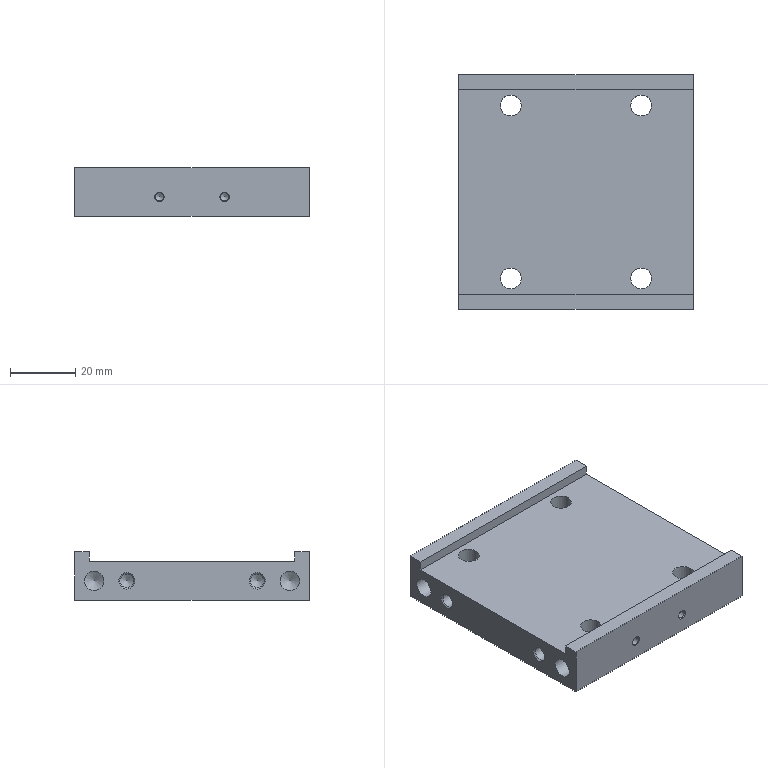Part | NX | 1 solid | 54 faces | box 72 x 72 x 15 mm | volume 58991 mm3 | cylinder 20 | cone 20 | plane 14 | commonest cylinder face diameters 2.5 x4 4.2 x4 6 x4 6.4 x4 11 x4
STEP:
#1=CARTESIAN_POINT('',(25.5,-26.5,0.));
#2=VERTEX_POINT('',#1);
#3=CARTESIAN_POINT('',(20.,-26.5,0.));
#4=DIRECTION('',(0.,0.,-1.));
#5=DIRECTION('',(1.,0.,0.));
#6=AXIS2_PLACEMENT_3D('',#3,#4,#5);
#7=CIRCLE('',#6,5.5);
#8=EDGE_CURVE('',#2,#2,#7,.T.);
#9=ORIENTED_EDGE('',*,*,#8,.F.);
#10=EDGE_LOOP('',(#9));
#11=FACE_BOUND('',#10,.T.);
#12=CARTESIAN_POINT('',(-36.,-36.,0.));
#13=VERTEX_POINT('',#12);
#14=CARTESIAN_POINT('',(-36.,36.,0.));
#15=VERTEX_POINT('',#14);
#16=CARTESIAN_POINT('',(-36.,-36.,0.));
#17=DIRECTION('',(0.,1.,0.));
#18=VECTOR('',#17,1.);
#19=LINE('',#16,#18);
#20=EDGE_CURVE('',#13,#15,#19,.T.);
#21=ORIENTED_EDGE('',*,*,#20,.T.);
#22=CARTESIAN_POINT('',(36.,36.,0.));
#23=VERTEX_POINT('',#22);
#24=CARTESIAN_POINT('',(36.,36.,0.));
#25=DIRECTION('',(-1.,0.,0.));
#26=VECTOR('',#25,1.);
#27=LINE('',#24,#26);
#28=EDGE_CURVE('',#23,#15,#27,.T.);
#29=ORIENTED_EDGE('',*,*,#28,.F.);
#30=CARTESIAN_POINT('',(36.,-36.,0.));
#31=VERTEX_POINT('',#30);
#32=CARTESIAN_POINT('',(36.,-36.,0.));
#33=DIRECTION('',(0.,1.,0.));
#34=VECTOR('',#33,1.);
#35=LINE('',#32,#34);
#36=EDGE_CURVE('',#31,#23,#35,.T.);
#37=ORIENTED_EDGE('',*,*,#36,.F.);
#38=CARTESIAN_POINT('',(36.,-36.,0.));
#39=DIRECTION('',(-1.,0.,0.));
#40=VECTOR('',#39,1.);
#41=LINE('',#38,#40);
#42=EDGE_CURVE('',#31,#13,#41,.T.);
#43=ORIENTED_EDGE('',*,*,#42,.T.);
#44=EDGE_LOOP('',(#21,#29,#37,#43));
#45=FACE_BOUND('',#44,.T.);
#46=CARTESIAN_POINT('',(-14.5,-26.5,0.));
#47=VERTEX_POINT('',#46);
#48=CARTESIAN_POINT('',(-20.,-26.5,0.));
#49=DIRECTION('',(0.,0.,1.));
#50=DIRECTION('',(1.,0.,0.));
#51=AXIS2_PLACEMENT_3D('',#48,#49,#50);
#52=CIRCLE('',#51,5.5);
#53=EDGE_CURVE('',#47,#47,#52,.T.);
#54=ORIENTED_EDGE('',*,*,#53,.T.);
#55=EDGE_LOOP('',(#54));
#56=FACE_BOUND('',#55,.T.);
#57=CARTESIAN_POINT('',(25.5,26.5,0.));
#58=VERTEX_POINT('',#57);
#59=CARTESIAN_POINT('',(20.,26.5,0.));
#60=DIRECTION('',(0.,0.,-1.));
#61=DIRECTION('',(1.,0.,0.));
#62=AXIS2_PLACEMENT_3D('',#59,#60,#61);
#63=CIRCLE('',#62,5.5);
#64=EDGE_CURVE('',#58,#58,#63,.T.);
#65=ORIENTED_EDGE('',*,*,#64,.F.);
#66=EDGE_LOOP('',(#65));
#67=FACE_BOUND('',#66,.T.);
#68=CARTESIAN_POINT('',(-14.5,26.5,0.));
#69=VERTEX_POINT('',#68);
#70=CARTESIAN_POINT('',(-20.,26.5,0.));
#71=DIRECTION('',(0.,0.,-1.));
#72=DIRECTION('',(1.,0.,0.));
#73=AXIS2_PLACEMENT_3D('',#70,#71,#72);
#74=CIRCLE('',#73,5.5);
#75=EDGE_CURVE('',#69,#69,#74,.T.);
#76=ORIENTED_EDGE('',*,*,#75,.F.);
#77=EDGE_LOOP('',(#76));
#78=FACE_BOUND('',#77,.T.);
#79=CARTESIAN_POINT('',(36.,-36.,0.));
#80=DIRECTION('',(0.,0.,1.));
#81=DIRECTION('',(-1.,0.,0.));
#82=AXIS2_PLACEMENT_3D('',#79,#80,#81);
#83=PLANE('',#82);
#84=ADVANCED_FACE('',(#11,#45,#56,#67,#78),#83,.F.);
#85=CARTESIAN_POINT('',(16.8,26.5,12.));
#86=VERTEX_POINT('',#85);
#87=CARTESIAN_POINT('',(20.,26.5,12.));
#88=DIRECTION('',(0.,0.,-1.));
#89=DIRECTION('',(-1.,0.,0.));
#90=AXIS2_PLACEMENT_3D('',#87,#88,#89);
#91=CIRCLE('',#90,3.2);
#92=EDGE_CURVE('',#86,#86,#91,.T.);
#93=ORIENTED_EDGE('',*,*,#92,.F.);
#94=EDGE_LOOP('',(#93));
#95=FACE_BOUND('',#94,.T.);
#96=CARTESIAN_POINT('',(16.8,26.5,6.8));
#97=VERTEX_POINT('',#96);
#98=CARTESIAN_POINT('',(20.,26.5,6.8));
#99=DIRECTION('',(0.,0.,1.));
#100=DIRECTION('',(-1.,0.,0.));
#101=AXIS2_PLACEMENT_3D('',#98,#99,#100);
#102=CIRCLE('',#101,3.2);
#103=EDGE_CURVE('',#97,#97,#102,.T.);
#104=ORIENTED_EDGE('',*,*,#103,.F.);
#105=EDGE_LOOP('',(#104));
#106=FACE_BOUND('',#105,.T.);
#107=CARTESIAN_POINT('',(20.,26.5,-60.));
#108=DIRECTION('',(0.,0.,1.));
#109=DIRECTION('',(-1.,0.,0.));
#110=AXIS2_PLACEMENT_3D('',#107,#108,#109);
#111=CYLINDRICAL_SURFACE('',#110,3.2);
#112=ADVANCED_FACE('',(#95,#106),#111,.F.);
#113=CARTESIAN_POINT('',(16.8,-26.5,12.));
#114=VERTEX_POINT('',#113);
#115=CARTESIAN_POINT('',(20.,-26.5,12.));
#116=DIRECTION('',(0.,0.,-1.));
#117=DIRECTION('',(-1.,0.,0.));
#118=AXIS2_PLACEMENT_3D('',#115,#116,#117);
#119=CIRCLE('',#118,3.2);
#120=EDGE_CURVE('',#114,#114,#119,.T.);
#121=ORIENTED_EDGE('',*,*,#120,.F.);
#122=EDGE_LOOP('',(#121));
#123=FACE_BOUND('',#122,.T.);
#124=CARTESIAN_POINT('',(16.8,-26.5,6.8));
#125=VERTEX_POINT('',#124);
#126=CARTESIAN_POINT('',(20.,-26.5,6.8));
#127=DIRECTION('',(0.,0.,1.));
#128=DIRECTION('',(-1.,0.,0.));
#129=AXIS2_PLACEMENT_3D('',#126,#127,#128);
#130=CIRCLE('',#129,3.2);
#131=EDGE_CURVE('',#125,#125,#130,.T.);
#132=ORIENTED_EDGE('',*,*,#131,.F.);
#133=EDGE_LOOP('',(#132));
#134=FACE_BOUND('',#133,.T.);
#135=CARTESIAN_POINT('',(20.,-26.5,-60.));
#136=DIRECTION('',(0.,0.,1.));
#137=DIRECTION('',(-1.,0.,0.));
#138=AXIS2_PLACEMENT_3D('',#135,#136,#137);
#139=CYLINDRICAL_SURFACE('',#138,3.2);
#140=ADVANCED_FACE('',(#123,#134),#139,.F.);
#141=CARTESIAN_POINT('',(-23.2,26.5,12.));
#142=VERTEX_POINT('',#141);
#143=CARTESIAN_POINT('',(-20.,26.5,12.));
#144=DIRECTION('',(0.,0.,-1.));
#145=DIRECTION('',(-1.,0.,0.));
#146=AXIS2_PLACEMENT_3D('',#143,#144,#145);
#147=CIRCLE('',#146,3.2);
#148=EDGE_CURVE('',#142,#142,#147,.T.);
#149=ORIENTED_EDGE('',*,*,#148,.F.);
#150=EDGE_LOOP('',(#149));
#151=FACE_BOUND('',#150,.T.);
#152=CARTESIAN_POINT('',(-23.2,26.5,6.8));
#153=VERTEX_POINT('',#152);
#154=CARTESIAN_POINT('',(-20.,26.5,6.8));
#155=DIRECTION('',(0.,0.,1.));
#156=DIRECTION('',(-1.,0.,0.));
#157=AXIS2_PLACEMENT_3D('',#154,#155,#156);
#158=CIRCLE('',#157,3.2);
#159=EDGE_CURVE('',#153,#153,#158,.T.);
#160=ORIENTED_EDGE('',*,*,#159,.F.);
#161=EDGE_LOOP('',(#160));
#162=FACE_BOUND('',#161,.T.);
#163=CARTESIAN_POINT('',(-20.,26.5,-60.));
#164=DIRECTION('',(0.,0.,1.));
#165=DIRECTION('',(-1.,0.,0.));
#166=AXIS2_PLACEMENT_3D('',#163,#164,#165);
#167=CYLINDRICAL_SURFACE('',#166,3.2);
#168=ADVANCED_FACE('',(#151,#162),#167,.F.);
#169=CARTESIAN_POINT('',(-23.2,-26.5,12.));
#170=VERTEX_POINT('',#169);
#171=CARTESIAN_POINT('',(-20.,-26.5,12.));
#172=DIRECTION('',(0.,0.,1.));
#173=DIRECTION('',(-1.,0.,0.));
#174=AXIS2_PLACEMENT_3D('',#171,#172,#173);
#175=CIRCLE('',#174,3.2);
#176=EDGE_CURVE('',#170,#170,#175,.T.);
#177=ORIENTED_EDGE('',*,*,#176,.F.);
#178=EDGE_LOOP('',(#177));
#179=FACE_BOUND('',#178,.T.);
#180=CARTESIAN_POINT('',(-36.,31.5,12.));
#181=VERTEX_POINT('',#180);
#182=CARTESIAN_POINT('',(-36.,-31.5,12.));
#183=VERTEX_POINT('',#182);
#184=CARTESIAN_POINT('',(-36.,31.5,12.));
#185=DIRECTION('',(0.,-1.,0.));
#186=VECTOR('',#185,1.);
#187=LINE('',#184,#186);
#188=EDGE_CURVE('',#181,#183,#187,.T.);
#189=ORIENTED_EDGE('',*,*,#188,.T.);
#190=CARTESIAN_POINT('',(36.,-31.5,12.));
#191=VERTEX_POINT('',#190);
#192=CARTESIAN_POINT('',(36.,-31.5,12.));
#193=DIRECTION('',(-1.,0.,0.));
#194=VECTOR('',#193,1.);
#195=LINE('',#192,#194);
#196=EDGE_CURVE('',#191,#183,#195,.T.);
#197=ORIENTED_EDGE('',*,*,#196,.F.);
#198=CARTESIAN_POINT('',(36.,31.5,12.));
#199=VERTEX_POINT('',#198);
#200=CARTESIAN_POINT('',(36.,31.5,12.));
#201=DIRECTION('',(0.,-1.,0.));
#202=VECTOR('',#201,1.);
#203=LINE('',#200,#202);
#204=EDGE_CURVE('',#199,#191,#203,.T.);
#205=ORIENTED_EDGE('',*,*,#204,.F.);
#206=CARTESIAN_POINT('',(36.,31.5,12.));
#207=DIRECTION('',(-1.,0.,0.));
#208=VECTOR('',#207,1.);
#209=LINE('',#206,#208);
#210=EDGE_CURVE('',#199,#181,#209,.T.);
#211=ORIENTED_EDGE('',*,*,#210,.T.);
#212=EDGE_LOOP('',(#189,#197,#205,#211));
#213=FACE_BOUND('',#212,.T.);
#214=ORIENTED_EDGE('',*,*,#92,.T.);
#215=EDGE_LOOP('',(#214));
#216=FACE_BOUND('',#215,.T.);
#217=ORIENTED_EDGE('',*,*,#120,.T.);
#218=EDGE_LOOP('',(#217));
#219=FACE_BOUND('',#218,.T.);
#220=ORIENTED_EDGE('',*,*,#148,.T.);
#221=EDGE_LOOP('',(#220));
#222=FACE_BOUND('',#221,.T.);
#223=CARTESIAN_POINT('',(36.,31.5,12.));
#224=DIRECTION('',(0.,0.,-1.));
#225=DIRECTION('',(1.,0.,0.));
#226=AXIS2_PLACEMENT_3D('',#223,#224,#225);
#227=PLANE('',#226);
#228=ADVANCED_FACE('',(#179,#213,#216,#219,#222),#227,.F.);
#229=CARTESIAN_POINT('',(10.,36.,4.5));
#230=VERTEX_POINT('',#229);
#231=CARTESIAN_POINT('',(10.,36.,6.));
#232=DIRECTION('',(0.,-1.,0.));
#233=DIRECTION('',(0.,0.,-1.));
#234=AXIS2_PLACEMENT_3D('',#231,#232,#233);
#235=CIRCLE('',#234,1.5);
#236=EDGE_CURVE('',#230,#230,#235,.T.);
#237=ORIENTED_EDGE('',*,*,#236,.T.);
#238=EDGE_LOOP('',(#237));
#239=FACE_BOUND('',#238,.T.);
#240=CARTESIAN_POINT('',(-10.,36.,4.5));
#241=VERTEX_POINT('',#240);
#242=CARTESIAN_POINT('',(-10.,36.,6.));
#243=DIRECTION('',(0.,-1.,0.));
#244=DIRECTION('',(0.,0.,-1.));
#245=AXIS2_PLACEMENT_3D('',#242,#243,#244);
#246=CIRCLE('',#245,1.5);
#247=EDGE_CURVE('',#241,#241,#246,.T.);
#248=ORIENTED_EDGE('',*,*,#247,.T.);
#249=EDGE_LOOP('',(#248));
#250=FACE_BOUND('',#249,.T.);
#251=CARTESIAN_POINT('',(-36.,36.,15.));
#252=VERTEX_POINT('',#251);
#253=CARTESIAN_POINT('',(-36.,36.,0.));
#254=DIRECTION('',(0.,0.,1.));
#255=VECTOR('',#254,1.);
#256=LINE('',#253,#255);
#257=EDGE_CURVE('',#15,#252,#256,.T.);
#258=ORIENTED_EDGE('',*,*,#257,.T.);
#259=CARTESIAN_POINT('',(36.,36.,15.));
#260=VERTEX_POINT('',#259);
#261=CARTESIAN_POINT('',(36.,36.,15.));
#262=DIRECTION('',(-1.,0.,0.));
#263=VECTOR('',#262,1.);
#264=LINE('',#261,#263);
#265=EDGE_CURVE('',#260,#252,#264,.T.);
#266=ORIENTED_EDGE('',*,*,#265,.F.);
#267=CARTESIAN_POINT('',(36.,36.,0.));
#268=DIRECTION('',(0.,0.,1.));
#269=VECTOR('',#268,1.);
#270=LINE('',#267,#269);
#271=EDGE_CURVE('',#23,#260,#270,.T.);
#272=ORIENTED_EDGE('',*,*,#271,.F.);
#273=ORIENTED_EDGE('',*,*,#28,.T.);
#274=EDGE_LOOP('',(#258,#266,#272,#273));
#275=FACE_BOUND('',#274,.T.);
#276=CARTESIAN_POINT('',(36.,36.,0.));
#277=DIRECTION('',(0.,-1.,0.));
#278=DIRECTION('',(0.,0.,1.));
#279=AXIS2_PLACEMENT_3D('',#276,#277,#278);
#280=PLANE('',#279);
#281=ADVANCED_FACE('',(#239,#250,#275),#280,.F.);
#282=CARTESIAN_POINT('',(-36.,31.5,15.));
#283=VERTEX_POINT('',#282);
#284=CARTESIAN_POINT('',(-36.,36.,15.));
#285=DIRECTION('',(0.,-1.,0.));
#286=VECTOR('',#285,1.);
#287=LINE('',#284,#286);
#288=EDGE_CURVE('',#252,#283,#287,.T.);
#289=ORIENTED_EDGE('',*,*,#288,.T.);
#290=CARTESIAN_POINT('',(36.,31.5,15.));
#291=VERTEX_POINT('',#290);
#292=CARTESIAN_POINT('',(36.,31.5,15.));
#293=DIRECTION('',(-1.,0.,0.));
#294=VECTOR('',#293,1.);
#295=LINE('',#292,#294);
#296=EDGE_CURVE('',#291,#283,#295,.T.);
#297=ORIENTED_EDGE('',*,*,#296,.F.);
#298=CARTESIAN_POINT('',(36.,36.,15.));
#299=DIRECTION('',(0.,-1.,0.));
#300=VECTOR('',#299,1.);
#301=LINE('',#298,#300);
#302=EDGE_CURVE('',#260,#291,#301,.T.);
#303=ORIENTED_EDGE('',*,*,#302,.F.);
#304=ORIENTED_EDGE('',*,*,#265,.T.);
#305=EDGE_LOOP('',(#289,#297,#303,#304));
#306=FACE_OUTER_BOUND('',#305,.T.);
#307=CARTESIAN_POINT('',(36.,36.,15.));
#308=DIRECTION('',(0.,0.,-1.));
#309=DIRECTION('',(1.,0.,0.));
#310=AXIS2_PLACEMENT_3D('',#307,#308,#309);
#311=PLANE('',#310);
#312=ADVANCED_FACE('',(#306),#311,.F.);
#313=CARTESIAN_POINT('',(-36.,31.5,15.));
#314=DIRECTION('',(0.,0.,-1.));
#315=VECTOR('',#314,1.);
#316=LINE('',#313,#315);
#317=EDGE_CURVE('',#283,#181,#316,.T.);
#318=ORIENTED_EDGE('',*,*,#317,.T.);
#319=ORIENTED_EDGE('',*,*,#210,.F.);
#320=CARTESIAN_POINT('',(36.,31.5,15.));
#321=DIRECTION('',(0.,0.,-1.));
#322=VECTOR('',#321,1.);
#323=LINE('',#320,#322);
#324=EDGE_CURVE('',#291,#199,#323,.T.);
#325=ORIENTED_EDGE('',*,*,#324,.F.);
#326=ORIENTED_EDGE('',*,*,#296,.T.);
#327=EDGE_LOOP('',(#318,#319,#325,#326));
#328=FACE_OUTER_BOUND('',#327,.T.);
#329=CARTESIAN_POINT('',(36.,31.5,15.));
#330=DIRECTION('',(0.,1.,0.));
#331=DIRECTION('',(0.,0.,-1.));
#332=AXIS2_PLACEMENT_3D('',#329,#330,#331);
#333=PLANE('',#332);
#334=ADVANCED_FACE('',(#328),#333,.F.);
#335=CARTESIAN_POINT('',(-36.,-31.5,15.));
#336=VERTEX_POINT('',#335);
#337=CARTESIAN_POINT('',(-36.,-31.5,12.));
#338=DIRECTION('',(0.,0.,1.));
#339=VECTOR('',#338,1.);
#340=LINE('',#337,#339);
#341=EDGE_CURVE('',#183,#336,#340,.T.);
#342=ORIENTED_EDGE('',*,*,#341,.T.);
#343=CARTESIAN_POINT('',(36.,-31.5,15.));
#344=VERTEX_POINT('',#343);
#345=CARTESIAN_POINT('',(36.,-31.5,15.));
#346=DIRECTION('',(-1.,0.,0.));
#347=VECTOR('',#346,1.);
#348=LINE('',#345,#347);
#349=EDGE_CURVE('',#344,#336,#348,.T.);
#350=ORIENTED_EDGE('',*,*,#349,.F.);
#351=CARTESIAN_POINT('',(36.,-31.5,12.));
#352=DIRECTION('',(0.,0.,1.));
#353=VECTOR('',#352,1.);
#354=LINE('',#351,#353);
#355=EDGE_CURVE('',#191,#344,#354,.T.);
#356=ORIENTED_EDGE('',*,*,#355,.F.);
#357=ORIENTED_EDGE('',*,*,#196,.T.);
#358=EDGE_LOOP('',(#342,#350,#356,#357));
#359=FACE_OUTER_BOUND('',#358,.T.);
#360=CARTESIAN_POINT('',(36.,-31.5,12.));
#361=DIRECTION('',(0.,-1.,0.));
#362=DIRECTION('',(0.,0.,1.));
#363=AXIS2_PLACEMENT_3D('',#360,#361,#362);
#364=PLANE('',#363);
#365=ADVANCED_FACE('',(#359),#364,.F.);
#366=CARTESIAN_POINT('',(-36.,-36.,15.));
#367=VERTEX_POINT('',#366);
#368=CARTESIAN_POINT('',(-36.,-31.5,15.));
#369=DIRECTION('',(0.,-1.,0.));
#370=VECTOR('',#369,1.);
#371=LINE('',#368,#370);
#372=EDGE_CURVE('',#336,#367,#371,.T.);
#373=ORIENTED_EDGE('',*,*,#372,.T.);
#374=CARTESIAN_POINT('',(36.,-36.,15.));
#375=VERTEX_POINT('',#374);
#376=CARTESIAN_POINT('',(36.,-36.,15.));
#377=DIRECTION('',(-1.,0.,0.));
#378=VECTOR('',#377,1.);
#379=LINE('',#376,#378);
#380=EDGE_CURVE('',#375,#367,#379,.T.);
#381=ORIENTED_EDGE('',*,*,#380,.F.);
#382=CARTESIAN_POINT('',(36.,-31.5,15.));
#383=DIRECTION('',(0.,-1.,0.));
#384=VECTOR('',#383,1.);
#385=LINE('',#382,#384);
#386=EDGE_CURVE('',#344,#375,#385,.T.);
#387=ORIENTED_EDGE('',*,*,#386,.F.);
#388=ORIENTED_EDGE('',*,*,#349,.T.);
#389=EDGE_LOOP('',(#373,#381,#387,#388));
#390=FACE_OUTER_BOUND('',#389,.T.);
#391=CARTESIAN_POINT('',(36.,-31.5,15.));
#392=DIRECTION('',(0.,0.,-1.));
#393=DIRECTION('',(1.,0.,0.));
#394=AXIS2_PLACEMENT_3D('',#391,#392,#393);
#395=PLANE('',#394);
#396=ADVANCED_FACE('',(#390),#395,.F.);
#397=CARTESIAN_POINT('',(10.,-36.,7.5));
#398=VERTEX_POINT('',#397);
#399=CARTESIAN_POINT('',(10.,-36.,6.));
#400=DIRECTION('',(0.,1.,0.));
#401=DIRECTION('',(0.,0.,1.));
#402=AXIS2_PLACEMENT_3D('',#399,#400,#401);
#403=CIRCLE('',#402,1.5);
#404=EDGE_CURVE('',#398,#398,#403,.T.);
#405=ORIENTED_EDGE('',*,*,#404,.T.);
#406=EDGE_LOOP('',(#405));
#407=FACE_BOUND('',#406,.T.);
#408=CARTESIAN_POINT('',(-10.,-36.,7.5));
#409=VERTEX_POINT('',#408);
#410=CARTESIAN_POINT('',(-10.,-36.,6.));
#411=DIRECTION('',(0.,1.,0.));
#412=DIRECTION('',(0.,0.,1.));
#413=AXIS2_PLACEMENT_3D('',#410,#411,#412);
#414=CIRCLE('',#413,1.5);
#415=EDGE_CURVE('',#409,#409,#414,.T.);
#416=ORIENTED_EDGE('',*,*,#415,.T.);
#417=EDGE_LOOP('',(#416));
#418=FACE_BOUND('',#417,.T.);
#419=CARTESIAN_POINT('',(-36.,-36.,15.));
#420=DIRECTION('',(0.,0.,-1.));
#421=VECTOR('',#420,1.);
#422=LINE('',#419,#421);
#423=EDGE_CURVE('',#367,#13,#422,.T.);
#424=ORIENTED_EDGE('',*,*,#423,.T.);
#425=ORIENTED_EDGE('',*,*,#42,.F.);
#426=CARTESIAN_POINT('',(36.,-36.,15.));
#427=DIRECTION('',(0.,0.,-1.));
#428=VECTOR('',#427,1.);
#429=LINE('',#426,#428);
#430=EDGE_CURVE('',#375,#31,#429,.T.);
#431=ORIENTED_EDGE('',*,*,#430,.F.);
#432=ORIENTED_EDGE('',*,*,#380,.T.);
#433=EDGE_LOOP('',(#424,#425,#431,#432));
#434=FACE_BOUND('',#433,.T.);
#435=CARTESIAN_POINT('',(36.,-36.,15.));
#436=DIRECTION('',(0.,1.,0.));
#437=DIRECTION('',(0.,0.,-1.));
#438=AXIS2_PLACEMENT_3D('',#435,#436,#437);
#439=PLANE('',#438);
#440=ADVANCED_FACE('',(#407,#418,#434),#439,.F.);
#441=CARTESIAN_POINT('',(36.,20.,3.5));
#442=VERTEX_POINT('',#441);
#443=CARTESIAN_POINT('',(36.,20.,6.));
#444=DIRECTION('',(-1.,0.,0.));
#445=DIRECTION('',(0.,0.,-1.));
#446=AXIS2_PLACEMENT_3D('',#443,#444,#445);
#447=CIRCLE('',#446,2.5);
#448=EDGE_CURVE('',#442,#442,#447,.T.);
#449=ORIENTED_EDGE('',*,*,#448,.T.);
#450=EDGE_LOOP('',(#449));
#451=FACE_BOUND('',#450,.T.);
#452=CARTESIAN_POINT('',(36.,-20.,3.5));
#453=VERTEX_POINT('',#452);
#454=CARTESIAN_POINT('',(36.,-20.,6.));
#455=DIRECTION('',(-1.,0.,0.));
#456=DIRECTION('',(0.,0.,-1.));
#457=AXIS2_PLACEMENT_3D('',#454,#455,#456);
#458=CIRCLE('',#457,2.5);
#459=EDGE_CURVE('',#453,#453,#458,.T.);
#460=ORIENTED_EDGE('',*,*,#459,.T.);
#461=EDGE_LOOP('',(#460));
#462=FACE_BOUND('',#461,.T.);
#463=CARTESIAN_POINT('',(36.,30.,9.));
#464=VERTEX_POINT('',#463);
#465=CARTESIAN_POINT('',(36.,30.,6.));
#466=DIRECTION('',(-1.,0.,0.));
#467=DIRECTION('',(0.,0.,1.));
#468=AXIS2_PLACEMENT_3D('',#465,#466,#467);
#469=CIRCLE('',#468,3.);
#470=EDGE_CURVE('',#464,#464,#469,.T.);
#471=ORIENTED_EDGE('',*,*,#470,.T.);
#472=EDGE_LOOP('',(#471));
#473=FACE_BOUND('',#472,.T.);
#474=CARTESIAN_POINT('',(36.,-30.,9.));
#475=VERTEX_POINT('',#474);
#476=CARTESIAN_POINT('',(36.,-30.,6.));
#477=DIRECTION('',(-1.,0.,0.));
#478=DIRECTION('',(0.,0.,1.));
#479=AXIS2_PLACEMENT_3D('',#476,#477,#478);
#480=CIRCLE('',#479,3.);
#481=EDGE_CURVE('',#475,#475,#480,.T.);
#482=ORIENTED_EDGE('',*,*,#481,.T.);
#483=EDGE_LOOP('',(#482));
#484=FACE_BOUND('',#483,.T.);
#485=ORIENTED_EDGE('',*,*,#36,.T.);
#486=ORIENTED_EDGE('',*,*,#271,.T.);
#487=ORIENTED_EDGE('',*,*,#302,.T.);
#488=ORIENTED_EDGE('',*,*,#324,.T.);
#489=ORIENTED_EDGE('',*,*,#204,.T.);
#490=ORIENTED_EDGE('',*,*,#355,.T.);
#491=ORIENTED_EDGE('',*,*,#386,.T.);
#492=ORIENTED_EDGE('',*,*,#430,.T.);
#493=EDGE_LOOP('',(#485,#486,#487,#488,#489,#490,#491,#492));
#494=FACE_BOUND('',#493,.T.);
#495=CARTESIAN_POINT('',(36.,0.,0.));
#496=DIRECTION('',(1.,0.,0.));
#497=DIRECTION('',(0.,0.,1.));
#498=AXIS2_PLACEMENT_3D('',#495,#496,#497);
#499=PLANE('',#498);
#500=ADVANCED_FACE('',(#451,#462,#473,#484,#494),#499,.T.);
#501=CARTESIAN_POINT('',(-36.,20.,3.5));
#502=VERTEX_POINT('',#501);
#503=CARTESIAN_POINT('',(-36.,20.,6.));
#504=DIRECTION('',(1.,0.,0.));
#505=DIRECTION('',(0.,0.,-1.));
#506=AXIS2_PLACEMENT_3D('',#503,#504,#505);
#507=CIRCLE('',#506,2.5);
#508=EDGE_CURVE('',#502,#502,#507,.T.);
#509=ORIENTED_EDGE('',*,*,#508,.T.);
#510=EDGE_LOOP('',(#509));
#511=FACE_BOUND('',#510,.T.);
#512=CARTESIAN_POINT('',(-36.,-20.,3.5));
#513=VERTEX_POINT('',#512);
#514=CARTESIAN_POINT('',(-36.,-20.,6.));
#515=DIRECTION('',(1.,0.,0.));
#516=DIRECTION('',(0.,0.,-1.));
#517=AXIS2_PLACEMENT_3D('',#514,#515,#516);
#518=CIRCLE('',#517,2.5);
#519=EDGE_CURVE('',#513,#513,#518,.T.);
#520=ORIENTED_EDGE('',*,*,#519,.T.);
#521=EDGE_LOOP('',(#520));
#522=FACE_BOUND('',#521,.T.);
#523=CARTESIAN_POINT('',(-36.,30.,3.));
#524=VERTEX_POINT('',#523);
#525=CARTESIAN_POINT('',(-36.,30.,6.));
#526=DIRECTION('',(1.,0.,0.));
#527=DIRECTION('',(0.,0.,-1.));
#528=AXIS2_PLACEMENT_3D('',#525,#526,#527);
#529=CIRCLE('',#528,3.);
#530=EDGE_CURVE('',#524,#524,#529,.T.);
#531=ORIENTED_EDGE('',*,*,#530,.T.);
#532=EDGE_LOOP('',(#531));
#533=FACE_BOUND('',#532,.T.);
#534=CARTESIAN_POINT('',(-36.,-30.,3.));
#535=VERTEX_POINT('',#534);
#536=CARTESIAN_POINT('',(-36.,-30.,6.));
#537=DIRECTION('',(1.,0.,0.));
#538=DIRECTION('',(0.,0.,-1.));
#539=AXIS2_PLACEMENT_3D('',#536,#537,#538);
#540=CIRCLE('',#539,3.);
#541=EDGE_CURVE('',#535,#535,#540,.T.);
#542=ORIENTED_EDGE('',*,*,#541,.T.);
#543=EDGE_LOOP('',(#542));
#544=FACE_BOUND('',#543,.T.);
#545=ORIENTED_EDGE('',*,*,#20,.F.);
#546=ORIENTED_EDGE('',*,*,#423,.F.);
#547=ORIENTED_EDGE('',*,*,#372,.F.);
#548=ORIENTED_EDGE('',*,*,#341,.F.);
#549=ORIENTED_EDGE('',*,*,#188,.F.);
#550=ORIENTED_EDGE('',*,*,#317,.F.);
#551=ORIENTED_EDGE('',*,*,#288,.F.);
#552=ORIENTED_EDGE('',*,*,#257,.F.);
#553=EDGE_LOOP('',(#545,#546,#547,#548,#549,#550,#551,#552));
#554=FACE_BOUND('',#553,.T.);
#555=CARTESIAN_POINT('',(-36.,0.,0.));
#556=DIRECTION('',(1.,0.,0.));
#557=DIRECTION('',(0.,0.,1.));
#558=AXIS2_PLACEMENT_3D('',#555,#556,#557);
#559=PLANE('',#558);
#560=ADVANCED_FACE('',(#511,#522,#533,#544,#554),#559,.F.);
#561=CARTESIAN_POINT('',(-16.8,-26.5,6.8));
#562=VERTEX_POINT('',#561);
#563=CARTESIAN_POINT('',(-20.,-26.5,6.8));
#564=DIRECTION('',(0.,0.,-1.));
#565=DIRECTION('',(1.,0.,0.));
#566=AXIS2_PLACEMENT_3D('',#563,#564,#565);
#567=CIRCLE('',#566,3.2);
#568=EDGE_CURVE('',#562,#562,#567,.T.);
#569=ORIENTED_EDGE('',*,*,#568,.T.);
#570=EDGE_LOOP('',(#569));
#571=FACE_BOUND('',#570,.T.);
#572=ORIENTED_EDGE('',*,*,#176,.T.);
#573=EDGE_LOOP('',(#572));
#574=FACE_BOUND('',#573,.T.);
#575=CARTESIAN_POINT('',(-20.,-26.5,-60.));
#576=DIRECTION('',(0.,0.,1.));
#577=DIRECTION('',(-1.,0.,0.));
#578=AXIS2_PLACEMENT_3D('',#575,#576,#577);
#579=CYLINDRICAL_SURFACE('',#578,3.2);
#580=ADVANCED_FACE('',(#571,#574),#579,.F.);
#581=CARTESIAN_POINT('',(-25.5,26.5,6.8));
#582=VERTEX_POINT('',#581);
#583=CARTESIAN_POINT('',(-20.,26.5,6.8));
#584=DIRECTION('',(0.,0.,-1.));
#585=DIRECTION('',(-1.,0.,0.));
#586=AXIS2_PLACEMENT_3D('',#583,#584,#585);
#587=CIRCLE('',#586,5.5);
#588=EDGE_CURVE('',#582,#582,#587,.T.);
#589=ORIENTED_EDGE('',*,*,#588,.F.);
#590=EDGE_LOOP('',(#589));
#591=FACE_BOUND('',#590,.T.);
#592=ORIENTED_EDGE('',*,*,#75,.T.);
#593=EDGE_LOOP('',(#592));
#594=FACE_BOUND('',#593,.T.);
#595=CARTESIAN_POINT('',(-20.,26.5,-60.));
#596=DIRECTION('',(0.,0.,1.));
#597=DIRECTION('',(-1.,0.,0.));
#598=AXIS2_PLACEMENT_3D('',#595,#596,#597);
#599=CYLINDRICAL_SURFACE('',#598,5.5);
#600=ADVANCED_FACE('',(#591,#594),#599,.F.);
#601=ORIENTED_EDGE('',*,*,#159,.T.);
#602=EDGE_LOOP('',(#601));
#603=FACE_BOUND('',#602,.T.);
#604=ORIENTED_EDGE('',*,*,#588,.T.);
#605=EDGE_LOOP('',(#604));
#606=FACE_BOUND('',#605,.T.);
#607=CARTESIAN_POINT('',(-20.,26.5,6.8));
#608=DIRECTION('',(0.,0.,-1.));
#609=DIRECTION('',(1.,0.,0.));
#610=AXIS2_PLACEMENT_3D('',#607,#608,#609);
#611=PLANE('',#610);
#612=ADVANCED_FACE('',(#603,#606),#611,.T.);
#613=CARTESIAN_POINT('',(14.5,-26.5,6.8));
#614=VERTEX_POINT('',#613);
#615=CARTESIAN_POINT('',(20.,-26.5,6.8));
#616=DIRECTION('',(0.,0.,-1.));
#617=DIRECTION('',(-1.,0.,0.));
#618=AXIS2_PLACEMENT_3D('',#615,#616,#617);
#619=CIRCLE('',#618,5.5);
#620=EDGE_CURVE('',#614,#614,#619,.T.);
#621=ORIENTED_EDGE('',*,*,#620,.F.);
#622=EDGE_LOOP('',(#621));
#623=FACE_BOUND('',#622,.T.);
#624=ORIENTED_EDGE('',*,*,#8,.T.);
#625=EDGE_LOOP('',(#624));
#626=FACE_BOUND('',#625,.T.);
#627=CARTESIAN_POINT('',(20.,-26.5,-60.));
#628=DIRECTION('',(0.,0.,1.));
#629=DIRECTION('',(-1.,0.,0.));
#630=AXIS2_PLACEMENT_3D('',#627,#628,#629);
#631=CYLINDRICAL_SURFACE('',#630,5.5);
#632=ADVANCED_FACE('',(#623,#626),#631,.F.);
#633=ORIENTED_EDGE('',*,*,#131,.T.);
#634=EDGE_LOOP('',(#633));
#635=FACE_BOUND('',#634,.T.);
#636=ORIENTED_EDGE('',*,*,#620,.T.);
#637=EDGE_LOOP('',(#636));
#638=FACE_BOUND('',#637,.T.);
#639=CARTESIAN_POINT('',(20.,-26.5,6.8));
#640=DIRECTION('',(0.,0.,-1.));
#641=DIRECTION('',(1.,0.,0.));
#642=AXIS2_PLACEMENT_3D('',#639,#640,#641);
#643=PLANE('',#642);
#644=ADVANCED_FACE('',(#635,#638),#643,.T.);
#645=CARTESIAN_POINT('',(14.5,26.5,6.8));
#646=VERTEX_POINT('',#645);
#647=CARTESIAN_POINT('',(20.,26.5,6.8));
#648=DIRECTION('',(0.,0.,-1.));
#649=DIRECTION('',(-1.,0.,0.));
#650=AXIS2_PLACEMENT_3D('',#647,#648,#649);
#651=CIRCLE('',#650,5.5);
#652=EDGE_CURVE('',#646,#646,#651,.T.);
#653=ORIENTED_EDGE('',*,*,#652,.F.);
#654=EDGE_LOOP('',(#653));
#655=FACE_BOUND('',#654,.T.);
#656=ORIENTED_EDGE('',*,*,#64,.T.);
#657=EDGE_LOOP('',(#656));
#658=FACE_BOUND('',#657,.T.);
#659=CARTESIAN_POINT('',(20.,26.5,-60.));
#660=DIRECTION('',(0.,0.,1.));
#661=DIRECTION('',(-1.,0.,0.));
#662=AXIS2_PLACEMENT_3D('',#659,#660,#661);
#663=CYLINDRICAL_SURFACE('',#662,5.5);
#664=ADVANCED_FACE('',(#655,#658),#663,.F.);
#665=ORIENTED_EDGE('',*,*,#103,.T.);
#666=EDGE_LOOP('',(#665));
#667=FACE_BOUND('',#666,.T.);
#668=ORIENTED_EDGE('',*,*,#652,.T.);
#669=EDGE_LOOP('',(#668));
#670=FACE_BOUND('',#669,.T.);
#671=CARTESIAN_POINT('',(20.,26.5,6.8));
#672=DIRECTION('',(0.,0.,-1.));
#673=DIRECTION('',(1.,0.,0.));
#674=AXIS2_PLACEMENT_3D('',#671,#672,#673);
#675=PLANE('',#674);
#676=ADVANCED_FACE('',(#667,#670),#675,.T.);
#677=CARTESIAN_POINT('',(-25.5,-26.5,6.8));
#678=VERTEX_POINT('',#677);
#679=CARTESIAN_POINT('',(-20.,-26.5,6.8));
#680=DIRECTION('',(0.,0.,1.));
#681=DIRECTION('',(-1.,0.,0.));
#682=AXIS2_PLACEMENT_3D('',#679,#680,#681);
#683=CIRCLE('',#682,5.5);
#684=EDGE_CURVE('',#678,#678,#683,.T.);
#685=ORIENTED_EDGE('',*,*,#684,.T.);
#686=EDGE_LOOP('',(#685));
#687=FACE_BOUND('',#686,.T.);
#688=ORIENTED_EDGE('',*,*,#53,.F.);
#689=EDGE_LOOP('',(#688));
#690=FACE_BOUND('',#689,.T.);
#691=CARTESIAN_POINT('',(-20.,-26.5,-60.));
#692=DIRECTION('',(0.,0.,1.));
#693=DIRECTION('',(-1.,0.,0.));
#694=AXIS2_PLACEMENT_3D('',#691,#692,#693);
#695=CYLINDRICAL_SURFACE('',#694,5.5);
#696=ADVANCED_FACE('',(#687,#690),#695,.F.);
#697=ORIENTED_EDGE('',*,*,#684,.F.);
#698=EDGE_LOOP('',(#697));
#699=FACE_BOUND('',#698,.T.);
#700=ORIENTED_EDGE('',*,*,#568,.F.);
#701=EDGE_LOOP('',(#700));
#702=FACE_BOUND('',#701,.T.);
#703=CARTESIAN_POINT('',(-20.,-26.5,6.8));
#704=DIRECTION('',(0.,0.,1.));
#705=DIRECTION('',(-1.,0.,0.));
#706=AXIS2_PLACEMENT_3D('',#703,#704,#705);
#707=PLANE('',#706);
#708=ADVANCED_FACE('',(#699,#702),#707,.F.);
#709=CARTESIAN_POINT('',(-28.,-30.,3.));
#710=VERTEX_POINT('',#709);
#711=CARTESIAN_POINT('',(-28.,-30.,6.));
#712=DIRECTION('',(-1.,0.,0.));
#713=DIRECTION('',(0.,0.,-1.));
#714=AXIS2_PLACEMENT_3D('',#711,#712,#713);
#715=CIRCLE('',#714,3.);
#716=EDGE_CURVE('',#710,#710,#715,.T.);
#717=ORIENTED_EDGE('',*,*,#716,.T.);
#718=EDGE_LOOP('',(#717));
#719=FACE_BOUND('',#718,.T.);
#720=CARTESIAN_POINT('',(-26.197,-30.,6.));
#721=VERTEX_POINT('',#720);
#722=VERTEX_LOOP('',#721);
#723=FACE_BOUND('',#722,.T.);
#724=CARTESIAN_POINT('',(-28.,-30.,6.));
#725=DIRECTION('',(-1.,0.,0.));
#726=DIRECTION('',(0.,0.,-1.));
#727=AXIS2_PLACEMENT_3D('',#724,#725,#726);
#728=CONICAL_SURFACE('',#727,3.,59.);
#729=ADVANCED_FACE('',(#719,#723),#728,.F.);
#730=ORIENTED_EDGE('',*,*,#716,.F.);
#731=EDGE_LOOP('',(#730));
#732=FACE_BOUND('',#731,.T.);
#733=ORIENTED_EDGE('',*,*,#541,.F.);
#734=EDGE_LOOP('',(#733));
#735=FACE_BOUND('',#734,.T.);
#736=CARTESIAN_POINT('',(-36.,-30.,6.));
#737=DIRECTION('',(1.,0.,0.));
#738=DIRECTION('',(0.,0.,1.));
#739=AXIS2_PLACEMENT_3D('',#736,#737,#738);
#740=CYLINDRICAL_SURFACE('',#739,3.);
#741=ADVANCED_FACE('',(#732,#735),#740,.F.);
#742=CARTESIAN_POINT('',(-28.,30.,3.));
#743=VERTEX_POINT('',#742);
#744=CARTESIAN_POINT('',(-28.,30.,6.));
#745=DIRECTION('',(-1.,0.,0.));
#746=DIRECTION('',(0.,0.,-1.));
#747=AXIS2_PLACEMENT_3D('',#744,#745,#746);
#748=CIRCLE('',#747,3.);
#749=EDGE_CURVE('',#743,#743,#748,.T.);
#750=ORIENTED_EDGE('',*,*,#749,.T.);
#751=EDGE_LOOP('',(#750));
#752=FACE_BOUND('',#751,.T.);
#753=CARTESIAN_POINT('',(-26.197,30.,6.));
#754=VERTEX_POINT('',#753);
#755=VERTEX_LOOP('',#754);
#756=FACE_BOUND('',#755,.T.);
#757=CARTESIAN_POINT('',(-28.,30.,6.));
#758=DIRECTION('',(-1.,0.,0.));
#759=DIRECTION('',(0.,0.,-1.));
#760=AXIS2_PLACEMENT_3D('',#757,#758,#759);
#761=CONICAL_SURFACE('',#760,3.,59.);
#762=ADVANCED_FACE('',(#752,#756),#761,.F.);
#763=ORIENTED_EDGE('',*,*,#749,.F.);
#764=EDGE_LOOP('',(#763));
#765=FACE_BOUND('',#764,.T.);
#766=ORIENTED_EDGE('',*,*,#530,.F.);
#767=EDGE_LOOP('',(#766));
#768=FACE_BOUND('',#767,.T.);
#769=CARTESIAN_POINT('',(-36.,30.,6.));
#770=DIRECTION('',(1.,0.,0.));
#771=DIRECTION('',(0.,0.,1.));
#772=AXIS2_PLACEMENT_3D('',#769,#770,#771);
#773=CYLINDRICAL_SURFACE('',#772,3.);
#774=ADVANCED_FACE('',(#765,#768),#773,.F.);
#775=CARTESIAN_POINT('',(-24.,-20.,3.9));
#776=VERTEX_POINT('',#775);
#777=CARTESIAN_POINT('',(-24.,-20.,6.));
#778=DIRECTION('',(-1.,0.,0.));
#779=DIRECTION('',(0.,0.,-1.));
#780=AXIS2_PLACEMENT_3D('',#777,#778,#779);
#781=CIRCLE('',#780,2.1);
#782=EDGE_CURVE('',#776,#776,#781,.T.);
#783=ORIENTED_EDGE('',*,*,#782,.T.);
#784=EDGE_LOOP('',(#783));
#785=FACE_BOUND('',#784,.T.);
#786=CARTESIAN_POINT('',(-22.738,-20.,6.));
#787=VERTEX_POINT('',#786);
#788=VERTEX_LOOP('',#787);
#789=FACE_BOUND('',#788,.T.);
#790=CARTESIAN_POINT('',(-24.,-20.,6.));
#791=DIRECTION('',(-1.,0.,0.));
#792=DIRECTION('',(0.,0.,-1.));
#793=AXIS2_PLACEMENT_3D('',#790,#791,#792);
#794=CONICAL_SURFACE('',#793,2.1,59.);
#795=ADVANCED_FACE('',(#785,#789),#794,.F.);
#796=CARTESIAN_POINT('',(-35.6,-20.,3.9));
#797=VERTEX_POINT('',#796);
#798=CARTESIAN_POINT('',(-35.6,-20.,6.));
#799=DIRECTION('',(-1.,0.,0.));
#800=DIRECTION('',(0.,0.,-1.));
#801=AXIS2_PLACEMENT_3D('',#798,#799,#800);
#802=CIRCLE('',#801,2.1);
#803=EDGE_CURVE('',#797,#797,#802,.T.);
#804=ORIENTED_EDGE('',*,*,#803,.T.);
#805=EDGE_LOOP('',(#804));
#806=FACE_BOUND('',#805,.T.);
#807=ORIENTED_EDGE('',*,*,#782,.F.);
#808=EDGE_LOOP('',(#807));
#809=FACE_BOUND('',#808,.T.);
#810=CARTESIAN_POINT('',(-36.,-20.,6.));
#811=DIRECTION('',(1.,0.,0.));
#812=DIRECTION('',(0.,0.,1.));
#813=AXIS2_PLACEMENT_3D('',#810,#811,#812);
#814=CYLINDRICAL_SURFACE('',#813,2.1);
#815=ADVANCED_FACE('',(#806,#809),#814,.F.);
#816=ORIENTED_EDGE('',*,*,#803,.F.);
#817=EDGE_LOOP('',(#816));
#818=FACE_BOUND('',#817,.T.);
#819=ORIENTED_EDGE('',*,*,#519,.F.);
#820=EDGE_LOOP('',(#819));
#821=FACE_BOUND('',#820,.T.);
#822=CARTESIAN_POINT('',(-36.,-20.,6.));
#823=DIRECTION('',(-1.,0.,0.));
#824=DIRECTION('',(0.,0.,-1.));
#825=AXIS2_PLACEMENT_3D('',#822,#823,#824);
#826=CONICAL_SURFACE('',#825,2.5,45.);
#827=ADVANCED_FACE('',(#818,#821),#826,.F.);
#828=CARTESIAN_POINT('',(-24.,20.,3.9));
#829=VERTEX_POINT('',#828);
#830=CARTESIAN_POINT('',(-24.,20.,6.));
#831=DIRECTION('',(-1.,0.,0.));
#832=DIRECTION('',(0.,0.,-1.));
#833=AXIS2_PLACEMENT_3D('',#830,#831,#832);
#834=CIRCLE('',#833,2.1);
#835=EDGE_CURVE('',#829,#829,#834,.T.);
#836=ORIENTED_EDGE('',*,*,#835,.T.);
#837=EDGE_LOOP('',(#836));
#838=FACE_BOUND('',#837,.T.);
#839=CARTESIAN_POINT('',(-22.738,20.,6.));
#840=VERTEX_POINT('',#839);
#841=VERTEX_LOOP('',#840);
#842=FACE_BOUND('',#841,.T.);
#843=CARTESIAN_POINT('',(-24.,20.,6.));
#844=DIRECTION('',(-1.,0.,0.));
#845=DIRECTION('',(0.,0.,-1.));
#846=AXIS2_PLACEMENT_3D('',#843,#844,#845);
#847=CONICAL_SURFACE('',#846,2.1,59.);
#848=ADVANCED_FACE('',(#838,#842),#847,.F.);
#849=CARTESIAN_POINT('',(-35.6,20.,3.9));
#850=VERTEX_POINT('',#849);
#851=CARTESIAN_POINT('',(-35.6,20.,6.));
#852=DIRECTION('',(-1.,0.,0.));
#853=DIRECTION('',(0.,0.,-1.));
#854=AXIS2_PLACEMENT_3D('',#851,#852,#853);
#855=CIRCLE('',#854,2.1);
#856=EDGE_CURVE('',#850,#850,#855,.T.);
#857=ORIENTED_EDGE('',*,*,#856,.T.);
#858=EDGE_LOOP('',(#857));
#859=FACE_BOUND('',#858,.T.);
#860=ORIENTED_EDGE('',*,*,#835,.F.);
#861=EDGE_LOOP('',(#860));
#862=FACE_BOUND('',#861,.T.);
#863=CARTESIAN_POINT('',(-36.,20.,6.));
#864=DIRECTION('',(1.,0.,0.));
#865=DIRECTION('',(0.,0.,1.));
#866=AXIS2_PLACEMENT_3D('',#863,#864,#865);
#867=CYLINDRICAL_SURFACE('',#866,2.1);
#868=ADVANCED_FACE('',(#859,#862),#867,.F.);
#869=ORIENTED_EDGE('',*,*,#856,.F.);
#870=EDGE_LOOP('',(#869));
#871=FACE_BOUND('',#870,.T.);
#872=ORIENTED_EDGE('',*,*,#508,.F.);
#873=EDGE_LOOP('',(#872));
#874=FACE_BOUND('',#873,.T.);
#875=CARTESIAN_POINT('',(-36.,20.,6.));
#876=DIRECTION('',(-1.,0.,0.));
#877=DIRECTION('',(0.,0.,-1.));
#878=AXIS2_PLACEMENT_3D('',#875,#876,#877);
#879=CONICAL_SURFACE('',#878,2.5,45.);
#880=ADVANCED_FACE('',(#871,#874),#879,.F.);
#881=CARTESIAN_POINT('',(-10.,24.,4.75));
#882=VERTEX_POINT('',#881);
#883=CARTESIAN_POINT('',(-10.,24.,6.));
#884=DIRECTION('',(0.,1.,0.));
#885=DIRECTION('',(0.,0.,-1.));
#886=AXIS2_PLACEMENT_3D('',#883,#884,#885);
#887=CIRCLE('',#886,1.25);
#888=EDGE_CURVE('',#882,#882,#887,.T.);
#889=ORIENTED_EDGE('',*,*,#888,.T.);
#890=EDGE_LOOP('',(#889));
#891=FACE_BOUND('',#890,.T.);
#892=CARTESIAN_POINT('',(-10.,23.249,6.));
#893=VERTEX_POINT('',#892);
#894=VERTEX_LOOP('',#893);
#895=FACE_BOUND('',#894,.T.);
#896=CARTESIAN_POINT('',(-10.,24.,6.));
#897=DIRECTION('',(0.,1.,0.));
#898=DIRECTION('',(0.,0.,-1.));
#899=AXIS2_PLACEMENT_3D('',#896,#897,#898);
#900=CONICAL_SURFACE('',#899,1.25,59.);
#901=ADVANCED_FACE('',(#891,#895),#900,.F.);
#902=CARTESIAN_POINT('',(-10.,35.75,4.75));
#903=VERTEX_POINT('',#902);
#904=CARTESIAN_POINT('',(-10.,35.75,6.));
#905=DIRECTION('',(0.,1.,0.));
#906=DIRECTION('',(0.,0.,-1.));
#907=AXIS2_PLACEMENT_3D('',#904,#905,#906);
#908=CIRCLE('',#907,1.25);
#909=EDGE_CURVE('',#903,#903,#908,.T.);
#910=ORIENTED_EDGE('',*,*,#909,.T.);
#911=EDGE_LOOP('',(#910));
#912=FACE_BOUND('',#911,.T.);
#913=ORIENTED_EDGE('',*,*,#888,.F.);
#914=EDGE_LOOP('',(#913));
#915=FACE_BOUND('',#914,.T.);
#916=CARTESIAN_POINT('',(-10.,36.,6.));
#917=DIRECTION('',(0.,-1.,0.));
#918=DIRECTION('',(0.,0.,1.));
#919=AXIS2_PLACEMENT_3D('',#916,#917,#918);
#920=CYLINDRICAL_SURFACE('',#919,1.25);
#921=ADVANCED_FACE('',(#912,#915),#920,.F.);
#922=ORIENTED_EDGE('',*,*,#909,.F.);
#923=EDGE_LOOP('',(#922));
#924=FACE_BOUND('',#923,.T.);
#925=ORIENTED_EDGE('',*,*,#247,.F.);
#926=EDGE_LOOP('',(#925));
#927=FACE_BOUND('',#926,.T.);
#928=CARTESIAN_POINT('',(-10.,36.,6.));
#929=DIRECTION('',(0.,1.,0.));
#930=DIRECTION('',(0.,0.,-1.));
#931=AXIS2_PLACEMENT_3D('',#928,#929,#930);
#932=CONICAL_SURFACE('',#931,1.5,45.);
#933=ADVANCED_FACE('',(#924,#927),#932,.F.);
#934=CARTESIAN_POINT('',(10.,24.,4.75));
#935=VERTEX_POINT('',#934);
#936=CARTESIAN_POINT('',(10.,24.,6.));
#937=DIRECTION('',(0.,1.,0.));
#938=DIRECTION('',(0.,0.,-1.));
#939=AXIS2_PLACEMENT_3D('',#936,#937,#938);
#940=CIRCLE('',#939,1.25);
#941=EDGE_CURVE('',#935,#935,#940,.T.);
#942=ORIENTED_EDGE('',*,*,#941,.T.);
#943=EDGE_LOOP('',(#942));
#944=FACE_BOUND('',#943,.T.);
#945=CARTESIAN_POINT('',(10.,23.249,6.));
#946=VERTEX_POINT('',#945);
#947=VERTEX_LOOP('',#946);
#948=FACE_BOUND('',#947,.T.);
#949=CARTESIAN_POINT('',(10.,24.,6.));
#950=DIRECTION('',(0.,1.,0.));
#951=DIRECTION('',(0.,0.,-1.));
#952=AXIS2_PLACEMENT_3D('',#949,#950,#951);
#953=CONICAL_SURFACE('',#952,1.25,59.);
#954=ADVANCED_FACE('',(#944,#948),#953,.F.);
#955=CARTESIAN_POINT('',(10.,35.75,4.75));
#956=VERTEX_POINT('',#955);
#957=CARTESIAN_POINT('',(10.,35.75,6.));
#958=DIRECTION('',(0.,1.,0.));
#959=DIRECTION('',(0.,0.,-1.));
#960=AXIS2_PLACEMENT_3D('',#957,#958,#959);
#961=CIRCLE('',#960,1.25);
#962=EDGE_CURVE('',#956,#956,#961,.T.);
#963=ORIENTED_EDGE('',*,*,#962,.T.);
#964=EDGE_LOOP('',(#963));
#965=FACE_BOUND('',#964,.T.);
#966=ORIENTED_EDGE('',*,*,#941,.F.);
#967=EDGE_LOOP('',(#966));
#968=FACE_BOUND('',#967,.T.);
#969=CARTESIAN_POINT('',(10.,36.,6.));
#970=DIRECTION('',(0.,-1.,0.));
#971=DIRECTION('',(0.,0.,1.));
#972=AXIS2_PLACEMENT_3D('',#969,#970,#971);
#973=CYLINDRICAL_SURFACE('',#972,1.25);
#974=ADVANCED_FACE('',(#965,#968),#973,.F.);
#975=ORIENTED_EDGE('',*,*,#962,.F.);
#976=EDGE_LOOP('',(#975));
#977=FACE_BOUND('',#976,.T.);
#978=ORIENTED_EDGE('',*,*,#236,.F.);
#979=EDGE_LOOP('',(#978));
#980=FACE_BOUND('',#979,.T.);
#981=CARTESIAN_POINT('',(10.,36.,6.));
#982=DIRECTION('',(0.,1.,0.));
#983=DIRECTION('',(0.,0.,-1.));
#984=AXIS2_PLACEMENT_3D('',#981,#982,#983);
#985=CONICAL_SURFACE('',#984,1.5,45.);
#986=ADVANCED_FACE('',(#977,#980),#985,.F.);
#987=CARTESIAN_POINT('',(-10.,-24.,7.25));
#988=VERTEX_POINT('',#987);
#989=CARTESIAN_POINT('',(-10.,-24.,6.));
#990=DIRECTION('',(0.,1.,0.));
#991=DIRECTION('',(0.,0.,1.));
#992=AXIS2_PLACEMENT_3D('',#989,#990,#991);
#993=CIRCLE('',#992,1.25);
#994=EDGE_CURVE('',#988,#988,#993,.T.);
#995=ORIENTED_EDGE('',*,*,#994,.F.);
#996=EDGE_LOOP('',(#995));
#997=FACE_BOUND('',#996,.T.);
#998=CARTESIAN_POINT('',(-10.,-23.249,6.));
#999=VERTEX_POINT('',#998);
#1000=VERTEX_LOOP('',#999);
#1001=FACE_BOUND('',#1000,.T.);
#1002=CARTESIAN_POINT('',(-10.,-24.,6.));
#1003=DIRECTION('',(0.,-1.,0.));
#1004=DIRECTION('',(0.,0.,1.));
#1005=AXIS2_PLACEMENT_3D('',#1002,#1003,#1004);
#1006=CONICAL_SURFACE('',#1005,1.25,59.);
#1007=ADVANCED_FACE('',(#997,#1001),#1006,.F.);
#1008=CARTESIAN_POINT('',(-10.,-35.75,7.25));
#1009=VERTEX_POINT('',#1008);
#1010=CARTESIAN_POINT('',(-10.,-35.75,6.));
#1011=DIRECTION('',(0.,1.,0.));
#1012=DIRECTION('',(0.,0.,1.));
#1013=AXIS2_PLACEMENT_3D('',#1010,#1011,#1012);
#1014=CIRCLE('',#1013,1.25);
#1015=EDGE_CURVE('',#1009,#1009,#1014,.T.);
#1016=ORIENTED_EDGE('',*,*,#1015,.F.);
#1017=EDGE_LOOP('',(#1016));
#1018=FACE_BOUND('',#1017,.T.);
#1019=ORIENTED_EDGE('',*,*,#994,.T.);
#1020=EDGE_LOOP('',(#1019));
#1021=FACE_BOUND('',#1020,.T.);
#1022=CARTESIAN_POINT('',(-10.,-36.,6.));
#1023=DIRECTION('',(0.,1.,0.));
#1024=DIRECTION('',(0.,0.,-1.));
#1025=AXIS2_PLACEMENT_3D('',#1022,#1023,#1024);
#1026=CYLINDRICAL_SURFACE('',#1025,1.25);
#1027=ADVANCED_FACE('',(#1018,#1021),#1026,.F.);
#1028=ORIENTED_EDGE('',*,*,#415,.F.);
#1029=EDGE_LOOP('',(#1028));
#1030=FACE_BOUND('',#1029,.T.);
#1031=ORIENTED_EDGE('',*,*,#1015,.T.);
#1032=EDGE_LOOP('',(#1031));
#1033=FACE_BOUND('',#1032,.T.);
#1034=CARTESIAN_POINT('',(-10.,-35.75,6.));
#1035=DIRECTION('',(0.,-1.,0.));
#1036=DIRECTION('',(0.,0.,1.));
#1037=AXIS2_PLACEMENT_3D('',#1034,#1035,#1036);
#1038=CONICAL_SURFACE('',#1037,1.25,45.);
#1039=ADVANCED_FACE('',(#1030,#1033),#1038,.F.);
#1040=CARTESIAN_POINT('',(10.,-24.,7.25));
#1041=VERTEX_POINT('',#1040);
#1042=CARTESIAN_POINT('',(10.,-24.,6.));
#1043=DIRECTION('',(0.,1.,0.));
#1044=DIRECTION('',(0.,0.,1.));
#1045=AXIS2_PLACEMENT_3D('',#1042,#1043,#1044);
#1046=CIRCLE('',#1045,1.25);
#1047=EDGE_CURVE('',#1041,#1041,#1046,.T.);
#1048=ORIENTED_EDGE('',*,*,#1047,.F.);
#1049=EDGE_LOOP('',(#1048));
#1050=FACE_BOUND('',#1049,.T.);
#1051=CARTESIAN_POINT('',(10.,-23.249,6.));
#1052=VERTEX_POINT('',#1051);
#1053=VERTEX_LOOP('',#1052);
#1054=FACE_BOUND('',#1053,.T.);
#1055=CARTESIAN_POINT('',(10.,-24.,6.));
#1056=DIRECTION('',(0.,-1.,0.));
#1057=DIRECTION('',(0.,0.,1.));
#1058=AXIS2_PLACEMENT_3D('',#1055,#1056,#1057);
#1059=CONICAL_SURFACE('',#1058,1.25,59.);
#1060=ADVANCED_FACE('',(#1050,#1054),#1059,.F.);
#1061=CARTESIAN_POINT('',(10.,-35.75,7.25));
#1062=VERTEX_POINT('',#1061);
#1063=CARTESIAN_POINT('',(10.,-35.75,6.));
#1064=DIRECTION('',(0.,1.,0.));
#1065=DIRECTION('',(0.,0.,1.));
#1066=AXIS2_PLACEMENT_3D('',#1063,#1064,#1065);
#1067=CIRCLE('',#1066,1.25);
#1068=EDGE_CURVE('',#1062,#1062,#1067,.T.);
#1069=ORIENTED_EDGE('',*,*,#1068,.F.);
#1070=EDGE_LOOP('',(#1069));
#1071=FACE_BOUND('',#1070,.T.);
#1072=ORIENTED_EDGE('',*,*,#1047,.T.);
#1073=EDGE_LOOP('',(#1072));
#1074=FACE_BOUND('',#1073,.T.);
#1075=CARTESIAN_POINT('',(10.,-36.,6.));
#1076=DIRECTION('',(0.,1.,0.));
#1077=DIRECTION('',(0.,0.,-1.));
#1078=AXIS2_PLACEMENT_3D('',#1075,#1076,#1077);
#1079=CYLINDRICAL_SURFACE('',#1078,1.25);
#1080=ADVANCED_FACE('',(#1071,#1074),#1079,.F.);
#1081=ORIENTED_EDGE('',*,*,#404,.F.);
#1082=EDGE_LOOP('',(#1081));
#1083=FACE_BOUND('',#1082,.T.);
#1084=ORIENTED_EDGE('',*,*,#1068,.T.);
#1085=EDGE_LOOP('',(#1084));
#1086=FACE_BOUND('',#1085,.T.);
#1087=CARTESIAN_POINT('',(10.,-35.75,6.));
#1088=DIRECTION('',(0.,-1.,0.));
#1089=DIRECTION('',(0.,0.,1.));
#1090=AXIS2_PLACEMENT_3D('',#1087,#1088,#1089);
#1091=CONICAL_SURFACE('',#1090,1.25,45.);
#1092=ADVANCED_FACE('',(#1083,#1086),#1091,.F.);
#1093=CARTESIAN_POINT('',(28.,-30.,9.));
#1094=VERTEX_POINT('',#1093);
#1095=CARTESIAN_POINT('',(28.,-30.,6.));
#1096=DIRECTION('',(-1.,0.,0.));
#1097=DIRECTION('',(0.,0.,1.));
#1098=AXIS2_PLACEMENT_3D('',#1095,#1096,#1097);
#1099=CIRCLE('',#1098,3.);
#1100=EDGE_CURVE('',#1094,#1094,#1099,.T.);
#1101=ORIENTED_EDGE('',*,*,#1100,.F.);
#1102=EDGE_LOOP('',(#1101));
#1103=FACE_BOUND('',#1102,.T.);
#1104=CARTESIAN_POINT('',(26.197,-30.,6.));
#1105=VERTEX_POINT('',#1104);
#1106=VERTEX_LOOP('',#1105);
#1107=FACE_BOUND('',#1106,.T.);
#1108=CARTESIAN_POINT('',(28.,-30.,6.));
#1109=DIRECTION('',(1.,0.,0.));
#1110=DIRECTION('',(0.,0.,1.));
#1111=AXIS2_PLACEMENT_3D('',#1108,#1109,#1110);
#1112=CONICAL_SURFACE('',#1111,3.,59.);
#1113=ADVANCED_FACE('',(#1103,#1107),#1112,.F.);
#1114=ORIENTED_EDGE('',*,*,#1100,.T.);
#1115=EDGE_LOOP('',(#1114));
#1116=FACE_BOUND('',#1115,.T.);
#1117=ORIENTED_EDGE('',*,*,#481,.F.);
#1118=EDGE_LOOP('',(#1117));
#1119=FACE_BOUND('',#1118,.T.);
#1120=CARTESIAN_POINT('',(36.,-30.,6.));
#1121=DIRECTION('',(-1.,0.,0.));
#1122=DIRECTION('',(0.,0.,-1.));
#1123=AXIS2_PLACEMENT_3D('',#1120,#1121,#1122);
#1124=CYLINDRICAL_SURFACE('',#1123,3.);
#1125=ADVANCED_FACE('',(#1116,#1119),#1124,.F.);
#1126=CARTESIAN_POINT('',(28.,30.,9.));
#1127=VERTEX_POINT('',#1126);
#1128=CARTESIAN_POINT('',(28.,30.,6.));
#1129=DIRECTION('',(-1.,0.,0.));
#1130=DIRECTION('',(0.,0.,1.));
#1131=AXIS2_PLACEMENT_3D('',#1128,#1129,#1130);
#1132=CIRCLE('',#1131,3.);
#1133=EDGE_CURVE('',#1127,#1127,#1132,.T.);
#1134=ORIENTED_EDGE('',*,*,#1133,.F.);
#1135=EDGE_LOOP('',(#1134));
#1136=FACE_BOUND('',#1135,.T.);
#1137=CARTESIAN_POINT('',(26.197,30.,6.));
#1138=VERTEX_POINT('',#1137);
#1139=VERTEX_LOOP('',#1138);
#1140=FACE_BOUND('',#1139,.T.);
#1141=CARTESIAN_POINT('',(28.,30.,6.));
#1142=DIRECTION('',(1.,0.,0.));
#1143=DIRECTION('',(0.,0.,1.));
#1144=AXIS2_PLACEMENT_3D('',#1141,#1142,#1143);
#1145=CONICAL_SURFACE('',#1144,3.,59.);
#1146=ADVANCED_FACE('',(#1136,#1140),#1145,.F.);
#1147=ORIENTED_EDGE('',*,*,#1133,.T.);
#1148=EDGE_LOOP('',(#1147));
#1149=FACE_BOUND('',#1148,.T.);
#1150=ORIENTED_EDGE('',*,*,#470,.F.);
#1151=EDGE_LOOP('',(#1150));
#1152=FACE_BOUND('',#1151,.T.);
#1153=CARTESIAN_POINT('',(36.,30.,6.));
#1154=DIRECTION('',(-1.,0.,0.));
#1155=DIRECTION('',(0.,0.,-1.));
#1156=AXIS2_PLACEMENT_3D('',#1153,#1154,#1155);
#1157=CYLINDRICAL_SURFACE('',#1156,3.);
#1158=ADVANCED_FACE('',(#1149,#1152),#1157,.F.);
#1159=CARTESIAN_POINT('',(24.,-20.,8.1));
#1160=VERTEX_POINT('',#1159);
#1161=CARTESIAN_POINT('',(24.,-20.,6.));
#1162=DIRECTION('',(-1.,0.,0.));
#1163=DIRECTION('',(0.,0.,1.));
#1164=AXIS2_PLACEMENT_3D('',#1161,#1162,#1163);
#1165=CIRCLE('',#1164,2.1);
#1166=EDGE_CURVE('',#1160,#1160,#1165,.T.);
#1167=ORIENTED_EDGE('',*,*,#1166,.F.);
#1168=EDGE_LOOP('',(#1167));
#1169=FACE_BOUND('',#1168,.T.);
#1170=CARTESIAN_POINT('',(22.738,-20.,6.));
#1171=VERTEX_POINT('',#1170);
#1172=VERTEX_LOOP('',#1171);
#1173=FACE_BOUND('',#1172,.T.);
#1174=CARTESIAN_POINT('',(24.,-20.,6.));
#1175=DIRECTION('',(1.,0.,0.));
#1176=DIRECTION('',(0.,0.,1.));
#1177=AXIS2_PLACEMENT_3D('',#1174,#1175,#1176);
#1178=CONICAL_SURFACE('',#1177,2.1,59.);
#1179=ADVANCED_FACE('',(#1169,#1173),#1178,.F.);
#1180=CARTESIAN_POINT('',(35.6,-20.,3.9));
#1181=VERTEX_POINT('',#1180);
#1182=CARTESIAN_POINT('',(35.6,-20.,6.));
#1183=DIRECTION('',(-1.,0.,0.));
#1184=DIRECTION('',(0.,0.,-1.));
#1185=AXIS2_PLACEMENT_3D('',#1182,#1183,#1184);
#1186=CIRCLE('',#1185,2.1);
#1187=EDGE_CURVE('',#1181,#1181,#1186,.T.);
#1188=ORIENTED_EDGE('',*,*,#1187,.F.);
#1189=EDGE_LOOP('',(#1188));
#1190=FACE_BOUND('',#1189,.T.);
#1191=ORIENTED_EDGE('',*,*,#1166,.T.);
#1192=EDGE_LOOP('',(#1191));
#1193=FACE_BOUND('',#1192,.T.);
#1194=CARTESIAN_POINT('',(36.,-20.,6.));
#1195=DIRECTION('',(-1.,0.,0.));
#1196=DIRECTION('',(0.,0.,-1.));
#1197=AXIS2_PLACEMENT_3D('',#1194,#1195,#1196);
#1198=CYLINDRICAL_SURFACE('',#1197,2.1);
#1199=ADVANCED_FACE('',(#1190,#1193),#1198,.F.);
#1200=ORIENTED_EDGE('',*,*,#1187,.T.);
#1201=EDGE_LOOP('',(#1200));
#1202=FACE_BOUND('',#1201,.T.);
#1203=ORIENTED_EDGE('',*,*,#459,.F.);
#1204=EDGE_LOOP('',(#1203));
#1205=FACE_BOUND('',#1204,.T.);
#1206=CARTESIAN_POINT('',(36.,-20.,6.));
#1207=DIRECTION('',(1.,0.,0.));
#1208=DIRECTION('',(0.,0.,1.));
#1209=AXIS2_PLACEMENT_3D('',#1206,#1207,#1208);
#1210=CONICAL_SURFACE('',#1209,2.5,45.);
#1211=ADVANCED_FACE('',(#1202,#1205),#1210,.F.);
#1212=CARTESIAN_POINT('',(24.,20.,8.1));
#1213=VERTEX_POINT('',#1212);
#1214=CARTESIAN_POINT('',(24.,20.,6.));
#1215=DIRECTION('',(-1.,0.,0.));
#1216=DIRECTION('',(0.,0.,1.));
#1217=AXIS2_PLACEMENT_3D('',#1214,#1215,#1216);
#1218=CIRCLE('',#1217,2.1);
#1219=EDGE_CURVE('',#1213,#1213,#1218,.T.);
#1220=ORIENTED_EDGE('',*,*,#1219,.F.);
#1221=EDGE_LOOP('',(#1220));
#1222=FACE_BOUND('',#1221,.T.);
#1223=CARTESIAN_POINT('',(22.738,20.,6.));
#1224=VERTEX_POINT('',#1223);
#1225=VERTEX_LOOP('',#1224);
#1226=FACE_BOUND('',#1225,.T.);
#1227=CARTESIAN_POINT('',(24.,20.,6.));
#1228=DIRECTION('',(1.,0.,0.));
#1229=DIRECTION('',(0.,0.,1.));
#1230=AXIS2_PLACEMENT_3D('',#1227,#1228,#1229);
#1231=CONICAL_SURFACE('',#1230,2.1,59.);
#1232=ADVANCED_FACE('',(#1222,#1226),#1231,.F.);
#1233=CARTESIAN_POINT('',(35.6,20.,3.9));
#1234=VERTEX_POINT('',#1233);
#1235=CARTESIAN_POINT('',(35.6,20.,6.));
#1236=DIRECTION('',(-1.,0.,0.));
#1237=DIRECTION('',(0.,0.,-1.));
#1238=AXIS2_PLACEMENT_3D('',#1235,#1236,#1237);
#1239=CIRCLE('',#1238,2.1);
#1240=EDGE_CURVE('',#1234,#1234,#1239,.T.);
#1241=ORIENTED_EDGE('',*,*,#1240,.F.);
#1242=EDGE_LOOP('',(#1241));
#1243=FACE_BOUND('',#1242,.T.);
#1244=ORIENTED_EDGE('',*,*,#1219,.T.);
#1245=EDGE_LOOP('',(#1244));
#1246=FACE_BOUND('',#1245,.T.);
#1247=CARTESIAN_POINT('',(36.,20.,6.));
#1248=DIRECTION('',(-1.,0.,0.));
#1249=DIRECTION('',(0.,0.,-1.));
#1250=AXIS2_PLACEMENT_3D('',#1247,#1248,#1249);
#1251=CYLINDRICAL_SURFACE('',#1250,2.1);
#1252=ADVANCED_FACE('',(#1243,#1246),#1251,.F.);
#1253=ORIENTED_EDGE('',*,*,#1240,.T.);
#1254=EDGE_LOOP('',(#1253));
#1255=FACE_BOUND('',#1254,.T.);
#1256=ORIENTED_EDGE('',*,*,#448,.F.);
#1257=EDGE_LOOP('',(#1256));
#1258=FACE_BOUND('',#1257,.T.);
#1259=CARTESIAN_POINT('',(36.,20.,6.));
#1260=DIRECTION('',(1.,0.,0.));
#1261=DIRECTION('',(0.,0.,1.));
#1262=AXIS2_PLACEMENT_3D('',#1259,#1260,#1261);
#1263=CONICAL_SURFACE('',#1262,2.5,45.);
#1264=ADVANCED_FACE('',(#1255,#1258),#1263,.F.);
#1265=CLOSED_SHELL('',(#84,#112,#140,#168,#228,#281,#312,#334,#365,#396,#440,#500,#560,#580,#600,#612,#632,#644,#664,#676,#696,#708,#729,#741,#762,#774,#795,#815,#827,#848,#868,#880,#901,#921,#933,#954,#974,#986,#1007,#1027,#1039,#1060,#1080,#1092,#1113,#1125,#1146,#1158,#1179,#1199,#1211,#1232,#1252,#1264));
#1266=MANIFOLD_SOLID_BREP('',#1265);
#1267=(LENGTH_UNIT()NAMED_UNIT(*)SI_UNIT(.MILLI.,.METRE.));
#1268=UNCERTAINTY_MEASURE_WITH_UNIT(LENGTH_MEASURE(0.00002),#1267,'','');
#1269=(NAMED_UNIT(*)PLANE_ANGLE_UNIT()SI_UNIT($,.RADIAN.));
#1270=PLANE_ANGLE_MEASURE_WITH_UNIT(PLANE_ANGLE_MEASURE(0.01745),#1269);
#1271=DIMENSIONAL_EXPONENTS(0.,0.,0.,0.,0.,0.,0.);
#1272=(CONVERSION_BASED_UNIT('DEGREE',#1270)NAMED_UNIT(#1271)PLANE_ANGLE_UNIT());
#1273=(NAMED_UNIT(*)SI_UNIT($,.STERADIAN.)SOLID_ANGLE_UNIT());
#1274=(GEOMETRIC_REPRESENTATION_CONTEXT(3)GLOBAL_UNCERTAINTY_ASSIGNED_CONTEXT((#1268))GLOBAL_UNIT_ASSIGNED_CONTEXT((#1267,#1272,#1273))REPRESENTATION_CONTEXT('',''));
#1275=ADVANCED_BREP_SHAPE_REPRESENTATION('',(#1266),#1274);